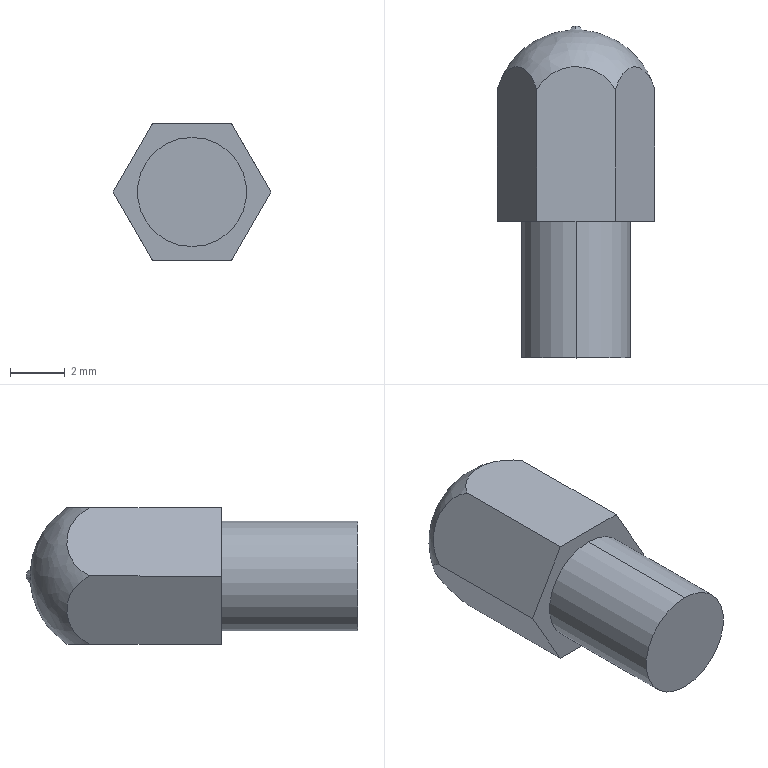Part | STEP file | 1 solid | 13 faces | box 5.774 x 12.16 x 5 mm | volume 199.597 mm3 | plane 8 | spline 3 | cylinder 2 | commonest cylinder face diameters 4 x2